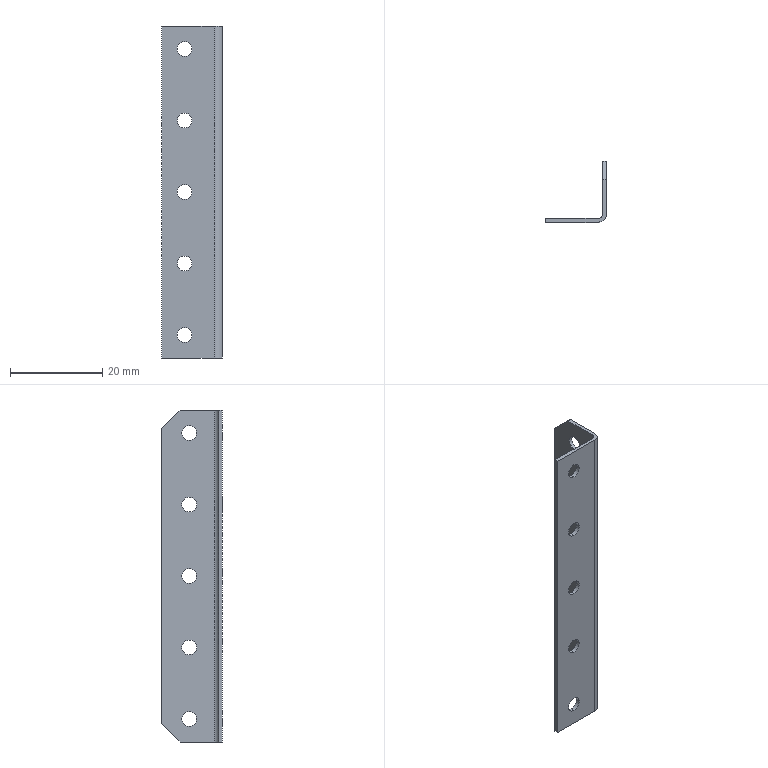Part | SolidWorks | features BaseBody 1 | 1 solid | 32 faces | box 13.2 x 13.2 x 72 mm | volume 1363 mm3 | cylinder 22 | plane 10 | commonest cylinder face diameters 3.2 x20 2 x1 3.6 x1
STEP:
#1=CARTESIAN_POINT('',(-7.5,-0.8,32.6));
#2=VERTEX_POINT('',#1);
#3=CARTESIAN_POINT('',(-7.5,-0.8,29.4));
#4=VERTEX_POINT('',#3);
#5=CARTESIAN_POINT('',(-7.5,-0.8,31.));
#6=DIRECTION('',(0.,-1.,0.));
#7=DIRECTION('',(0.,0.,1.));
#8=AXIS2_PLACEMENT_3D('',#5,#6,#7);
#9=CIRCLE('',#8,1.6);
#10=EDGE_CURVE('',#2,#4,#9,.T.);
#11=ORIENTED_EDGE('',*,*,#10,.T.);
#12=CARTESIAN_POINT('',(-7.5,0.,29.4));
#13=VERTEX_POINT('',#12);
#14=CARTESIAN_POINT('',(-7.5,-0.8,29.4));
#15=DIRECTION('',(0.,1.,0.));
#16=VECTOR('',#15,1000.);
#17=LINE('',#14,#16);
#18=EDGE_CURVE('',#4,#13,#17,.T.);
#19=ORIENTED_EDGE('',*,*,#18,.T.);
#20=CARTESIAN_POINT('',(-7.5,0.,32.6));
#21=VERTEX_POINT('',#20);
#22=CARTESIAN_POINT('',(-7.5,0.,31.));
#23=DIRECTION('',(0.,1.,0.));
#24=DIRECTION('',(0.,0.,1.));
#25=AXIS2_PLACEMENT_3D('',#22,#23,#24);
#26=CIRCLE('',#25,1.6);
#27=EDGE_CURVE('',#13,#21,#26,.T.);
#28=ORIENTED_EDGE('',*,*,#27,.T.);
#29=CARTESIAN_POINT('',(-7.5,-0.8,32.6));
#30=DIRECTION('',(0.,1.,0.));
#31=VECTOR('',#30,1000.);
#32=LINE('',#29,#31);
#33=EDGE_CURVE('',#2,#21,#32,.T.);
#34=ORIENTED_EDGE('',*,*,#33,.F.);
#35=EDGE_LOOP('',(#11,#19,#28,#34));
#36=FACE_OUTER_BOUND('',#35,.T.);
#37=CARTESIAN_POINT('',(-7.5,-0.8,31.));
#38=DIRECTION('',(0.,1.,0.));
#39=DIRECTION('',(0.,0.,1.));
#40=AXIS2_PLACEMENT_3D('',#37,#38,#39);
#41=CYLINDRICAL_SURFACE('',#40,1.6);
#42=ADVANCED_FACE('',(#36),#41,.F.);
#43=CARTESIAN_POINT('',(-7.5,-0.8,-32.6));
#44=VERTEX_POINT('',#43);
#45=CARTESIAN_POINT('',(-7.5,-0.8,-29.4));
#46=VERTEX_POINT('',#45);
#47=CARTESIAN_POINT('',(-7.5,-0.8,-31.));
#48=DIRECTION('',(0.,1.,0.));
#49=DIRECTION('',(0.,0.,1.));
#50=AXIS2_PLACEMENT_3D('',#47,#48,#49);
#51=CIRCLE('',#50,1.6);
#52=EDGE_CURVE('',#44,#46,#51,.T.);
#53=ORIENTED_EDGE('',*,*,#52,.F.);
#54=CARTESIAN_POINT('',(-7.5,0.,-32.6));
#55=VERTEX_POINT('',#54);
#56=CARTESIAN_POINT('',(-7.5,-0.8,-32.6));
#57=DIRECTION('',(0.,1.,0.));
#58=VECTOR('',#57,1000.);
#59=LINE('',#56,#58);
#60=EDGE_CURVE('',#44,#55,#59,.T.);
#61=ORIENTED_EDGE('',*,*,#60,.T.);
#62=CARTESIAN_POINT('',(-7.5,0.,-29.4));
#63=VERTEX_POINT('',#62);
#64=CARTESIAN_POINT('',(-7.5,0.,-31.));
#65=DIRECTION('',(0.,1.,0.));
#66=DIRECTION('',(0.,0.,1.));
#67=AXIS2_PLACEMENT_3D('',#64,#65,#66);
#68=CIRCLE('',#67,1.6);
#69=EDGE_CURVE('',#55,#63,#68,.T.);
#70=ORIENTED_EDGE('',*,*,#69,.T.);
#71=CARTESIAN_POINT('',(-7.5,-0.8,-29.4));
#72=DIRECTION('',(0.,1.,0.));
#73=VECTOR('',#72,1000.);
#74=LINE('',#71,#73);
#75=EDGE_CURVE('',#46,#63,#74,.T.);
#76=ORIENTED_EDGE('',*,*,#75,.F.);
#77=EDGE_LOOP('',(#53,#61,#70,#76));
#78=FACE_OUTER_BOUND('',#77,.T.);
#79=CARTESIAN_POINT('',(-7.5,-0.8,-31.));
#80=DIRECTION('',(0.,1.,0.));
#81=DIRECTION('',(0.,0.,1.));
#82=AXIS2_PLACEMENT_3D('',#79,#80,#81);
#83=CYLINDRICAL_SURFACE('',#82,1.6);
#84=ADVANCED_FACE('',(#78),#83,.F.);
#85=CARTESIAN_POINT('',(-7.5,-0.8,-1.6));
#86=VERTEX_POINT('',#85);
#87=CARTESIAN_POINT('',(-7.5,-0.8,1.6));
#88=VERTEX_POINT('',#87);
#89=CARTESIAN_POINT('',(-7.5,-0.8,0.));
#90=DIRECTION('',(0.,1.,0.));
#91=DIRECTION('',(0.,0.,1.));
#92=AXIS2_PLACEMENT_3D('',#89,#90,#91);
#93=CIRCLE('',#92,1.6);
#94=EDGE_CURVE('',#86,#88,#93,.T.);
#95=ORIENTED_EDGE('',*,*,#94,.F.);
#96=CARTESIAN_POINT('',(-7.5,0.,-1.6));
#97=VERTEX_POINT('',#96);
#98=CARTESIAN_POINT('',(-7.5,-0.8,-1.6));
#99=DIRECTION('',(0.,1.,0.));
#100=VECTOR('',#99,1000.);
#101=LINE('',#98,#100);
#102=EDGE_CURVE('',#86,#97,#101,.T.);
#103=ORIENTED_EDGE('',*,*,#102,.T.);
#104=CARTESIAN_POINT('',(-7.5,0.,1.6));
#105=VERTEX_POINT('',#104);
#106=CARTESIAN_POINT('',(-7.5,0.,0.));
#107=DIRECTION('',(0.,1.,0.));
#108=DIRECTION('',(0.,0.,1.));
#109=AXIS2_PLACEMENT_3D('',#106,#107,#108);
#110=CIRCLE('',#109,1.6);
#111=EDGE_CURVE('',#97,#105,#110,.T.);
#112=ORIENTED_EDGE('',*,*,#111,.T.);
#113=CARTESIAN_POINT('',(-7.5,-0.8,1.6));
#114=DIRECTION('',(0.,1.,0.));
#115=VECTOR('',#114,1000.);
#116=LINE('',#113,#115);
#117=EDGE_CURVE('',#88,#105,#116,.T.);
#118=ORIENTED_EDGE('',*,*,#117,.F.);
#119=EDGE_LOOP('',(#95,#103,#112,#118));
#120=FACE_OUTER_BOUND('',#119,.T.);
#121=CARTESIAN_POINT('',(-7.5,-0.8,0.));
#122=DIRECTION('',(0.,1.,0.));
#123=DIRECTION('',(0.,0.,1.));
#124=AXIS2_PLACEMENT_3D('',#121,#122,#123);
#125=CYLINDRICAL_SURFACE('',#124,1.6);
#126=ADVANCED_FACE('',(#120),#125,.F.);
#127=CARTESIAN_POINT('',(-7.5,-0.8,-17.1));
#128=VERTEX_POINT('',#127);
#129=CARTESIAN_POINT('',(-7.5,-0.8,-13.9));
#130=VERTEX_POINT('',#129);
#131=CARTESIAN_POINT('',(-7.5,-0.8,-15.5));
#132=DIRECTION('',(0.,1.,0.));
#133=DIRECTION('',(0.,0.,1.));
#134=AXIS2_PLACEMENT_3D('',#131,#132,#133);
#135=CIRCLE('',#134,1.6);
#136=EDGE_CURVE('',#128,#130,#135,.T.);
#137=ORIENTED_EDGE('',*,*,#136,.F.);
#138=CARTESIAN_POINT('',(-7.5,0.,-17.1));
#139=VERTEX_POINT('',#138);
#140=CARTESIAN_POINT('',(-7.5,-0.8,-17.1));
#141=DIRECTION('',(0.,1.,0.));
#142=VECTOR('',#141,1000.);
#143=LINE('',#140,#142);
#144=EDGE_CURVE('',#128,#139,#143,.T.);
#145=ORIENTED_EDGE('',*,*,#144,.T.);
#146=CARTESIAN_POINT('',(-7.5,0.,-13.9));
#147=VERTEX_POINT('',#146);
#148=CARTESIAN_POINT('',(-7.5,0.,-15.5));
#149=DIRECTION('',(0.,1.,0.));
#150=DIRECTION('',(0.,0.,1.));
#151=AXIS2_PLACEMENT_3D('',#148,#149,#150);
#152=CIRCLE('',#151,1.6);
#153=EDGE_CURVE('',#139,#147,#152,.T.);
#154=ORIENTED_EDGE('',*,*,#153,.T.);
#155=CARTESIAN_POINT('',(-7.5,-0.8,-13.9));
#156=DIRECTION('',(0.,1.,0.));
#157=VECTOR('',#156,1000.);
#158=LINE('',#155,#157);
#159=EDGE_CURVE('',#130,#147,#158,.T.);
#160=ORIENTED_EDGE('',*,*,#159,.F.);
#161=EDGE_LOOP('',(#137,#145,#154,#160));
#162=FACE_OUTER_BOUND('',#161,.T.);
#163=CARTESIAN_POINT('',(-7.5,-0.8,-15.5));
#164=DIRECTION('',(0.,1.,0.));
#165=DIRECTION('',(0.,0.,1.));
#166=AXIS2_PLACEMENT_3D('',#163,#164,#165);
#167=CYLINDRICAL_SURFACE('',#166,1.6);
#168=ADVANCED_FACE('',(#162),#167,.F.);
#169=CARTESIAN_POINT('',(-7.5,-0.8,13.9));
#170=VERTEX_POINT('',#169);
#171=CARTESIAN_POINT('',(-7.5,-0.8,17.1));
#172=VERTEX_POINT('',#171);
#173=CARTESIAN_POINT('',(-7.5,-0.8,15.5));
#174=DIRECTION('',(0.,1.,0.));
#175=DIRECTION('',(0.,0.,1.));
#176=AXIS2_PLACEMENT_3D('',#173,#174,#175);
#177=CIRCLE('',#176,1.6);
#178=EDGE_CURVE('',#170,#172,#177,.T.);
#179=ORIENTED_EDGE('',*,*,#178,.F.);
#180=CARTESIAN_POINT('',(-7.5,0.,13.9));
#181=VERTEX_POINT('',#180);
#182=CARTESIAN_POINT('',(-7.5,-0.8,13.9));
#183=DIRECTION('',(0.,1.,0.));
#184=VECTOR('',#183,1000.);
#185=LINE('',#182,#184);
#186=EDGE_CURVE('',#170,#181,#185,.T.);
#187=ORIENTED_EDGE('',*,*,#186,.T.);
#188=CARTESIAN_POINT('',(-7.5,0.,17.1));
#189=VERTEX_POINT('',#188);
#190=CARTESIAN_POINT('',(-7.5,0.,15.5));
#191=DIRECTION('',(0.,1.,0.));
#192=DIRECTION('',(0.,0.,1.));
#193=AXIS2_PLACEMENT_3D('',#190,#191,#192);
#194=CIRCLE('',#193,1.6);
#195=EDGE_CURVE('',#181,#189,#194,.T.);
#196=ORIENTED_EDGE('',*,*,#195,.T.);
#197=CARTESIAN_POINT('',(-7.5,-0.8,17.1));
#198=DIRECTION('',(0.,1.,0.));
#199=VECTOR('',#198,1000.);
#200=LINE('',#197,#199);
#201=EDGE_CURVE('',#172,#189,#200,.T.);
#202=ORIENTED_EDGE('',*,*,#201,.F.);
#203=EDGE_LOOP('',(#179,#187,#196,#202));
#204=FACE_OUTER_BOUND('',#203,.T.);
#205=CARTESIAN_POINT('',(-7.5,-0.8,15.5));
#206=DIRECTION('',(0.,1.,0.));
#207=DIRECTION('',(0.,0.,1.));
#208=AXIS2_PLACEMENT_3D('',#205,#206,#207);
#209=CYLINDRICAL_SURFACE('',#208,1.6);
#210=ADVANCED_FACE('',(#204),#209,.F.);
#211=CARTESIAN_POINT('',(0.7004,6.4,-32.6));
#212=VERTEX_POINT('',#211);
#213=CARTESIAN_POINT('',(0.7004,6.4,-29.4));
#214=VERTEX_POINT('',#213);
#215=CARTESIAN_POINT('',(0.7004,6.4,-31.));
#216=DIRECTION('',(-1.,0.,0.));
#217=DIRECTION('',(0.,0.,1.));
#218=AXIS2_PLACEMENT_3D('',#215,#216,#217);
#219=CIRCLE('',#218,1.6);
#220=EDGE_CURVE('',#212,#214,#219,.T.);
#221=ORIENTED_EDGE('',*,*,#220,.F.);
#222=CARTESIAN_POINT('',(-0.09956,6.4,-32.6));
#223=VERTEX_POINT('',#222);
#224=CARTESIAN_POINT('',(0.7004,6.4,-32.6));
#225=DIRECTION('',(-1.,0.,0.));
#226=VECTOR('',#225,1000.);
#227=LINE('',#224,#226);
#228=EDGE_CURVE('',#212,#223,#227,.T.);
#229=ORIENTED_EDGE('',*,*,#228,.T.);
#230=CARTESIAN_POINT('',(-0.09956,6.4,-29.4));
#231=VERTEX_POINT('',#230);
#232=CARTESIAN_POINT('',(-0.09956,6.4,-31.));
#233=DIRECTION('',(-1.,0.,0.));
#234=DIRECTION('',(0.,0.,1.));
#235=AXIS2_PLACEMENT_3D('',#232,#233,#234);
#236=CIRCLE('',#235,1.6);
#237=EDGE_CURVE('',#223,#231,#236,.T.);
#238=ORIENTED_EDGE('',*,*,#237,.T.);
#239=CARTESIAN_POINT('',(0.7004,6.4,-29.4));
#240=DIRECTION('',(-1.,0.,0.));
#241=VECTOR('',#240,1000.);
#242=LINE('',#239,#241);
#243=EDGE_CURVE('',#214,#231,#242,.T.);
#244=ORIENTED_EDGE('',*,*,#243,.F.);
#245=EDGE_LOOP('',(#221,#229,#238,#244));
#246=FACE_OUTER_BOUND('',#245,.T.);
#247=CARTESIAN_POINT('',(0.7004,6.4,-31.));
#248=DIRECTION('',(-1.,0.,0.));
#249=DIRECTION('',(0.,0.,1.));
#250=AXIS2_PLACEMENT_3D('',#247,#248,#249);
#251=CYLINDRICAL_SURFACE('',#250,1.6);
#252=ADVANCED_FACE('',(#246),#251,.F.);
#253=CARTESIAN_POINT('',(0.7004,6.4,29.4));
#254=VERTEX_POINT('',#253);
#255=CARTESIAN_POINT('',(0.7004,6.4,32.6));
#256=VERTEX_POINT('',#255);
#257=CARTESIAN_POINT('',(0.7004,6.4,31.));
#258=DIRECTION('',(-1.,0.,0.));
#259=DIRECTION('',(0.,0.,1.));
#260=AXIS2_PLACEMENT_3D('',#257,#258,#259);
#261=CIRCLE('',#260,1.6);
#262=EDGE_CURVE('',#254,#256,#261,.T.);
#263=ORIENTED_EDGE('',*,*,#262,.F.);
#264=CARTESIAN_POINT('',(-0.09956,6.4,29.4));
#265=VERTEX_POINT('',#264);
#266=CARTESIAN_POINT('',(0.7004,6.4,29.4));
#267=DIRECTION('',(-1.,0.,0.));
#268=VECTOR('',#267,1000.);
#269=LINE('',#266,#268);
#270=EDGE_CURVE('',#254,#265,#269,.T.);
#271=ORIENTED_EDGE('',*,*,#270,.T.);
#272=CARTESIAN_POINT('',(-0.09956,6.4,32.6));
#273=VERTEX_POINT('',#272);
#274=CARTESIAN_POINT('',(-0.09956,6.4,31.));
#275=DIRECTION('',(-1.,0.,0.));
#276=DIRECTION('',(0.,0.,1.));
#277=AXIS2_PLACEMENT_3D('',#274,#275,#276);
#278=CIRCLE('',#277,1.6);
#279=EDGE_CURVE('',#265,#273,#278,.T.);
#280=ORIENTED_EDGE('',*,*,#279,.T.);
#281=CARTESIAN_POINT('',(0.7004,6.4,32.6));
#282=DIRECTION('',(-1.,0.,0.));
#283=VECTOR('',#282,1000.);
#284=LINE('',#281,#283);
#285=EDGE_CURVE('',#256,#273,#284,.T.);
#286=ORIENTED_EDGE('',*,*,#285,.F.);
#287=EDGE_LOOP('',(#263,#271,#280,#286));
#288=FACE_OUTER_BOUND('',#287,.T.);
#289=CARTESIAN_POINT('',(0.7004,6.4,31.));
#290=DIRECTION('',(-1.,0.,0.));
#291=DIRECTION('',(0.,0.,1.));
#292=AXIS2_PLACEMENT_3D('',#289,#290,#291);
#293=CYLINDRICAL_SURFACE('',#292,1.6);
#294=ADVANCED_FACE('',(#288),#293,.F.);
#295=CARTESIAN_POINT('',(0.7004,6.4,-1.6));
#296=VERTEX_POINT('',#295);
#297=CARTESIAN_POINT('',(0.7004,6.4,1.6));
#298=VERTEX_POINT('',#297);
#299=CARTESIAN_POINT('',(0.7004,6.4,0.));
#300=DIRECTION('',(-1.,0.,0.));
#301=DIRECTION('',(0.,0.,1.));
#302=AXIS2_PLACEMENT_3D('',#299,#300,#301);
#303=CIRCLE('',#302,1.6);
#304=EDGE_CURVE('',#296,#298,#303,.T.);
#305=ORIENTED_EDGE('',*,*,#304,.F.);
#306=CARTESIAN_POINT('',(-0.09956,6.4,-1.6));
#307=VERTEX_POINT('',#306);
#308=CARTESIAN_POINT('',(0.7004,6.4,-1.6));
#309=DIRECTION('',(-1.,0.,0.));
#310=VECTOR('',#309,1000.);
#311=LINE('',#308,#310);
#312=EDGE_CURVE('',#296,#307,#311,.T.);
#313=ORIENTED_EDGE('',*,*,#312,.T.);
#314=CARTESIAN_POINT('',(-0.09956,6.4,1.6));
#315=VERTEX_POINT('',#314);
#316=CARTESIAN_POINT('',(-0.09956,6.4,0.));
#317=DIRECTION('',(-1.,0.,0.));
#318=DIRECTION('',(0.,0.,1.));
#319=AXIS2_PLACEMENT_3D('',#316,#317,#318);
#320=CIRCLE('',#319,1.6);
#321=EDGE_CURVE('',#307,#315,#320,.T.);
#322=ORIENTED_EDGE('',*,*,#321,.T.);
#323=CARTESIAN_POINT('',(0.7004,6.4,1.6));
#324=DIRECTION('',(-1.,0.,0.));
#325=VECTOR('',#324,1000.);
#326=LINE('',#323,#325);
#327=EDGE_CURVE('',#298,#315,#326,.T.);
#328=ORIENTED_EDGE('',*,*,#327,.F.);
#329=EDGE_LOOP('',(#305,#313,#322,#328));
#330=FACE_OUTER_BOUND('',#329,.T.);
#331=CARTESIAN_POINT('',(0.7004,6.4,0.));
#332=DIRECTION('',(-1.,0.,0.));
#333=DIRECTION('',(0.,0.,1.));
#334=AXIS2_PLACEMENT_3D('',#331,#332,#333);
#335=CYLINDRICAL_SURFACE('',#334,1.6);
#336=ADVANCED_FACE('',(#330),#335,.F.);
#337=CARTESIAN_POINT('',(0.7004,6.4,13.9));
#338=VERTEX_POINT('',#337);
#339=CARTESIAN_POINT('',(0.7004,6.4,17.1));
#340=VERTEX_POINT('',#339);
#341=CARTESIAN_POINT('',(0.7004,6.4,15.5));
#342=DIRECTION('',(-1.,0.,0.));
#343=DIRECTION('',(0.,0.,1.));
#344=AXIS2_PLACEMENT_3D('',#341,#342,#343);
#345=CIRCLE('',#344,1.6);
#346=EDGE_CURVE('',#338,#340,#345,.T.);
#347=ORIENTED_EDGE('',*,*,#346,.F.);
#348=CARTESIAN_POINT('',(-0.09956,6.4,13.9));
#349=VERTEX_POINT('',#348);
#350=CARTESIAN_POINT('',(0.7004,6.4,13.9));
#351=DIRECTION('',(-1.,0.,0.));
#352=VECTOR('',#351,1000.);
#353=LINE('',#350,#352);
#354=EDGE_CURVE('',#338,#349,#353,.T.);
#355=ORIENTED_EDGE('',*,*,#354,.T.);
#356=CARTESIAN_POINT('',(-0.09956,6.4,17.1));
#357=VERTEX_POINT('',#356);
#358=CARTESIAN_POINT('',(-0.09956,6.4,15.5));
#359=DIRECTION('',(-1.,0.,0.));
#360=DIRECTION('',(0.,0.,1.));
#361=AXIS2_PLACEMENT_3D('',#358,#359,#360);
#362=CIRCLE('',#361,1.6);
#363=EDGE_CURVE('',#349,#357,#362,.T.);
#364=ORIENTED_EDGE('',*,*,#363,.T.);
#365=CARTESIAN_POINT('',(0.7004,6.4,17.1));
#366=DIRECTION('',(-1.,0.,0.));
#367=VECTOR('',#366,1000.);
#368=LINE('',#365,#367);
#369=EDGE_CURVE('',#340,#357,#368,.T.);
#370=ORIENTED_EDGE('',*,*,#369,.F.);
#371=EDGE_LOOP('',(#347,#355,#364,#370));
#372=FACE_OUTER_BOUND('',#371,.T.);
#373=CARTESIAN_POINT('',(0.7004,6.4,15.5));
#374=DIRECTION('',(-1.,0.,0.));
#375=DIRECTION('',(0.,0.,1.));
#376=AXIS2_PLACEMENT_3D('',#373,#374,#375);
#377=CYLINDRICAL_SURFACE('',#376,1.6);
#378=ADVANCED_FACE('',(#372),#377,.F.);
#379=CARTESIAN_POINT('',(0.7004,6.4,-17.1));
#380=VERTEX_POINT('',#379);
#381=CARTESIAN_POINT('',(0.7004,6.4,-13.9));
#382=VERTEX_POINT('',#381);
#383=CARTESIAN_POINT('',(0.7004,6.4,-15.5));
#384=DIRECTION('',(-1.,0.,0.));
#385=DIRECTION('',(0.,0.,1.));
#386=AXIS2_PLACEMENT_3D('',#383,#384,#385);
#387=CIRCLE('',#386,1.6);
#388=EDGE_CURVE('',#380,#382,#387,.T.);
#389=ORIENTED_EDGE('',*,*,#388,.F.);
#390=CARTESIAN_POINT('',(-0.09956,6.4,-17.1));
#391=VERTEX_POINT('',#390);
#392=CARTESIAN_POINT('',(0.7004,6.4,-17.1));
#393=DIRECTION('',(-1.,0.,0.));
#394=VECTOR('',#393,1000.);
#395=LINE('',#392,#394);
#396=EDGE_CURVE('',#380,#391,#395,.T.);
#397=ORIENTED_EDGE('',*,*,#396,.T.);
#398=CARTESIAN_POINT('',(-0.09956,6.4,-13.9));
#399=VERTEX_POINT('',#398);
#400=CARTESIAN_POINT('',(-0.09956,6.4,-15.5));
#401=DIRECTION('',(-1.,0.,0.));
#402=DIRECTION('',(0.,0.,1.));
#403=AXIS2_PLACEMENT_3D('',#400,#401,#402);
#404=CIRCLE('',#403,1.6);
#405=EDGE_CURVE('',#391,#399,#404,.T.);
#406=ORIENTED_EDGE('',*,*,#405,.T.);
#407=CARTESIAN_POINT('',(0.7004,6.4,-13.9));
#408=DIRECTION('',(-1.,0.,0.));
#409=VECTOR('',#408,1000.);
#410=LINE('',#407,#409);
#411=EDGE_CURVE('',#382,#399,#410,.T.);
#412=ORIENTED_EDGE('',*,*,#411,.F.);
#413=EDGE_LOOP('',(#389,#397,#406,#412));
#414=FACE_OUTER_BOUND('',#413,.T.);
#415=CARTESIAN_POINT('',(0.7004,6.4,-15.5));
#416=DIRECTION('',(-1.,0.,0.));
#417=DIRECTION('',(0.,0.,1.));
#418=AXIS2_PLACEMENT_3D('',#415,#416,#417);
#419=CYLINDRICAL_SURFACE('',#418,1.6);
#420=ADVANCED_FACE('',(#414),#419,.F.);
#421=ORIENTED_EDGE('',*,*,#18,.F.);
#422=CARTESIAN_POINT('',(-7.5,-0.8,31.));
#423=DIRECTION('',(0.,-1.,0.));
#424=DIRECTION('',(0.,0.,1.));
#425=AXIS2_PLACEMENT_3D('',#422,#423,#424);
#426=CIRCLE('',#425,1.6);
#427=EDGE_CURVE('',#4,#2,#426,.T.);
#428=ORIENTED_EDGE('',*,*,#427,.T.);
#429=ORIENTED_EDGE('',*,*,#33,.T.);
#430=CARTESIAN_POINT('',(-7.5,0.,31.));
#431=DIRECTION('',(0.,1.,0.));
#432=DIRECTION('',(0.,0.,1.));
#433=AXIS2_PLACEMENT_3D('',#430,#431,#432);
#434=CIRCLE('',#433,1.6);
#435=EDGE_CURVE('',#21,#13,#434,.T.);
#436=ORIENTED_EDGE('',*,*,#435,.T.);
#437=EDGE_LOOP('',(#421,#428,#429,#436));
#438=FACE_OUTER_BOUND('',#437,.T.);
#439=CARTESIAN_POINT('',(-7.5,-0.8,31.));
#440=DIRECTION('',(0.,1.,0.));
#441=DIRECTION('',(0.,0.,1.));
#442=AXIS2_PLACEMENT_3D('',#439,#440,#441);
#443=CYLINDRICAL_SURFACE('',#442,1.6);
#444=ADVANCED_FACE('',(#438),#443,.F.);
#445=CARTESIAN_POINT('',(-7.5,0.,-31.));
#446=DIRECTION('',(0.,1.,0.));
#447=DIRECTION('',(0.,0.,1.));
#448=AXIS2_PLACEMENT_3D('',#445,#446,#447);
#449=CIRCLE('',#448,1.6);
#450=EDGE_CURVE('',#63,#55,#449,.T.);
#451=ORIENTED_EDGE('',*,*,#450,.F.);
#452=ORIENTED_EDGE('',*,*,#69,.F.);
#453=EDGE_LOOP('',(#451,#452));
#454=FACE_BOUND('',#453,.T.);
#455=CARTESIAN_POINT('',(-7.5,0.,0.));
#456=DIRECTION('',(0.,1.,0.));
#457=DIRECTION('',(0.,0.,1.));
#458=AXIS2_PLACEMENT_3D('',#455,#456,#457);
#459=CIRCLE('',#458,1.6);
#460=EDGE_CURVE('',#105,#97,#459,.T.);
#461=ORIENTED_EDGE('',*,*,#460,.F.);
#462=ORIENTED_EDGE('',*,*,#111,.F.);
#463=EDGE_LOOP('',(#461,#462));
#464=FACE_BOUND('',#463,.T.);
#465=CARTESIAN_POINT('',(-7.5,0.,-15.5));
#466=DIRECTION('',(0.,1.,0.));
#467=DIRECTION('',(0.,0.,1.));
#468=AXIS2_PLACEMENT_3D('',#465,#466,#467);
#469=CIRCLE('',#468,1.6);
#470=EDGE_CURVE('',#147,#139,#469,.T.);
#471=ORIENTED_EDGE('',*,*,#470,.F.);
#472=ORIENTED_EDGE('',*,*,#153,.F.);
#473=EDGE_LOOP('',(#471,#472));
#474=FACE_BOUND('',#473,.T.);
#475=CARTESIAN_POINT('',(-7.5,0.,15.5));
#476=DIRECTION('',(0.,1.,0.));
#477=DIRECTION('',(0.,0.,1.));
#478=AXIS2_PLACEMENT_3D('',#475,#476,#477);
#479=CIRCLE('',#478,1.6);
#480=EDGE_CURVE('',#189,#181,#479,.T.);
#481=ORIENTED_EDGE('',*,*,#480,.F.);
#482=ORIENTED_EDGE('',*,*,#195,.F.);
#483=EDGE_LOOP('',(#481,#482));
#484=FACE_BOUND('',#483,.T.);
#485=ORIENTED_EDGE('',*,*,#435,.F.);
#486=ORIENTED_EDGE('',*,*,#27,.F.);
#487=EDGE_LOOP('',(#485,#486));
#488=FACE_BOUND('',#487,.T.);
#489=CARTESIAN_POINT('',(-12.5,0.,-36.));
#490=VERTEX_POINT('',#489);
#491=CARTESIAN_POINT('',(-1.1,0.,-36.));
#492=VERTEX_POINT('',#491);
#493=CARTESIAN_POINT('',(-6.8,0.,-36.));
#494=DIRECTION('',(1.,0.,0.));
#495=VECTOR('',#494,1000.);
#496=LINE('',#493,#495);
#497=EDGE_CURVE('',#490,#492,#496,.T.);
#498=ORIENTED_EDGE('',*,*,#497,.F.);
#499=CARTESIAN_POINT('',(-12.5,0.,36.));
#500=VERTEX_POINT('',#499);
#501=CARTESIAN_POINT('',(-12.5,0.,0.));
#502=DIRECTION('',(0.,0.,-1.));
#503=VECTOR('',#502,1000.);
#504=LINE('',#501,#503);
#505=EDGE_CURVE('',#500,#490,#504,.T.);
#506=ORIENTED_EDGE('',*,*,#505,.F.);
#507=CARTESIAN_POINT('',(-1.1,0.,36.));
#508=VERTEX_POINT('',#507);
#509=CARTESIAN_POINT('',(-6.8,0.,36.));
#510=DIRECTION('',(-1.,0.,0.));
#511=VECTOR('',#510,1000.);
#512=LINE('',#509,#511);
#513=EDGE_CURVE('',#508,#500,#512,.T.);
#514=ORIENTED_EDGE('',*,*,#513,.F.);
#515=CARTESIAN_POINT('',(-1.1,0.,0.));
#516=DIRECTION('',(0.,0.,1.));
#517=VECTOR('',#516,1000.);
#518=LINE('',#515,#517);
#519=EDGE_CURVE('',#492,#508,#518,.T.);
#520=ORIENTED_EDGE('',*,*,#519,.F.);
#521=EDGE_LOOP('',(#498,#506,#514,#520));
#522=FACE_OUTER_BOUND('',#521,.T.);
#523=CARTESIAN_POINT('',(-12.5,0.,36.));
#524=DIRECTION('',(0.,-1.,0.));
#525=DIRECTION('',(0.,0.,-1.));
#526=AXIS2_PLACEMENT_3D('',#523,#524,#525);
#527=PLANE('',#526);
#528=ADVANCED_FACE('',(#454,#464,#474,#484,#488,#522),#527,.F.);
#529=CARTESIAN_POINT('',(-7.5,-0.8,-31.));
#530=DIRECTION('',(0.,1.,0.));
#531=DIRECTION('',(0.,0.,1.));
#532=AXIS2_PLACEMENT_3D('',#529,#530,#531);
#533=CIRCLE('',#532,1.6);
#534=EDGE_CURVE('',#46,#44,#533,.T.);
#535=ORIENTED_EDGE('',*,*,#534,.T.);
#536=ORIENTED_EDGE('',*,*,#52,.T.);
#537=EDGE_LOOP('',(#535,#536));
#538=FACE_BOUND('',#537,.T.);
#539=CARTESIAN_POINT('',(-7.5,-0.8,0.));
#540=DIRECTION('',(0.,1.,0.));
#541=DIRECTION('',(0.,0.,1.));
#542=AXIS2_PLACEMENT_3D('',#539,#540,#541);
#543=CIRCLE('',#542,1.6);
#544=EDGE_CURVE('',#88,#86,#543,.T.);
#545=ORIENTED_EDGE('',*,*,#544,.T.);
#546=ORIENTED_EDGE('',*,*,#94,.T.);
#547=EDGE_LOOP('',(#545,#546));
#548=FACE_BOUND('',#547,.T.);
#549=CARTESIAN_POINT('',(-7.5,-0.8,-15.5));
#550=DIRECTION('',(0.,1.,0.));
#551=DIRECTION('',(0.,0.,1.));
#552=AXIS2_PLACEMENT_3D('',#549,#550,#551);
#553=CIRCLE('',#552,1.6);
#554=EDGE_CURVE('',#130,#128,#553,.T.);
#555=ORIENTED_EDGE('',*,*,#554,.T.);
#556=ORIENTED_EDGE('',*,*,#136,.T.);
#557=EDGE_LOOP('',(#555,#556));
#558=FACE_BOUND('',#557,.T.);
#559=CARTESIAN_POINT('',(-7.5,-0.8,15.5));
#560=DIRECTION('',(0.,1.,0.));
#561=DIRECTION('',(0.,0.,1.));
#562=AXIS2_PLACEMENT_3D('',#559,#560,#561);
#563=CIRCLE('',#562,1.6);
#564=EDGE_CURVE('',#172,#170,#563,.T.);
#565=ORIENTED_EDGE('',*,*,#564,.T.);
#566=ORIENTED_EDGE('',*,*,#178,.T.);
#567=EDGE_LOOP('',(#565,#566));
#568=FACE_BOUND('',#567,.T.);
#569=ORIENTED_EDGE('',*,*,#10,.F.);
#570=ORIENTED_EDGE('',*,*,#427,.F.);
#571=EDGE_LOOP('',(#569,#570));
#572=FACE_BOUND('',#571,.T.);
#573=CARTESIAN_POINT('',(-1.1,-0.8,36.));
#574=VERTEX_POINT('',#573);
#575=CARTESIAN_POINT('',(-12.5,-0.8,36.));
#576=VERTEX_POINT('',#575);
#577=CARTESIAN_POINT('',(-6.8,-0.8,36.));
#578=DIRECTION('',(-1.,0.,0.));
#579=VECTOR('',#578,1000.);
#580=LINE('',#577,#579);
#581=EDGE_CURVE('',#574,#576,#580,.T.);
#582=ORIENTED_EDGE('',*,*,#581,.T.);
#583=CARTESIAN_POINT('',(-12.5,-0.8,-36.));
#584=VERTEX_POINT('',#583);
#585=CARTESIAN_POINT('',(-12.5,-0.8,0.));
#586=DIRECTION('',(0.,0.,-1.));
#587=VECTOR('',#586,1000.);
#588=LINE('',#585,#587);
#589=EDGE_CURVE('',#576,#584,#588,.T.);
#590=ORIENTED_EDGE('',*,*,#589,.T.);
#591=CARTESIAN_POINT('',(-1.1,-0.8,-36.));
#592=VERTEX_POINT('',#591);
#593=CARTESIAN_POINT('',(-6.8,-0.8,-36.));
#594=DIRECTION('',(1.,0.,0.));
#595=VECTOR('',#594,1000.);
#596=LINE('',#593,#595);
#597=EDGE_CURVE('',#584,#592,#596,.T.);
#598=ORIENTED_EDGE('',*,*,#597,.T.);
#599=CARTESIAN_POINT('',(-1.1,-0.8,0.));
#600=DIRECTION('',(0.,0.,1.));
#601=VECTOR('',#600,1000.);
#602=LINE('',#599,#601);
#603=EDGE_CURVE('',#592,#574,#602,.T.);
#604=ORIENTED_EDGE('',*,*,#603,.T.);
#605=EDGE_LOOP('',(#582,#590,#598,#604));
#606=FACE_OUTER_BOUND('',#605,.T.);
#607=CARTESIAN_POINT('',(-12.5,-0.8,36.));
#608=DIRECTION('',(0.,-1.,0.));
#609=DIRECTION('',(0.,0.,-1.));
#610=AXIS2_PLACEMENT_3D('',#607,#608,#609);
#611=PLANE('',#610);
#612=ADVANCED_FACE('',(#538,#548,#558,#568,#572,#606),#611,.T.);
#613=ORIENTED_EDGE('',*,*,#60,.F.);
#614=ORIENTED_EDGE('',*,*,#534,.F.);
#615=ORIENTED_EDGE('',*,*,#75,.T.);
#616=ORIENTED_EDGE('',*,*,#450,.T.);
#617=EDGE_LOOP('',(#613,#614,#615,#616));
#618=FACE_OUTER_BOUND('',#617,.T.);
#619=CARTESIAN_POINT('',(-7.5,-0.8,-31.));
#620=DIRECTION('',(0.,1.,0.));
#621=DIRECTION('',(0.,0.,1.));
#622=AXIS2_PLACEMENT_3D('',#619,#620,#621);
#623=CYLINDRICAL_SURFACE('',#622,1.6);
#624=ADVANCED_FACE('',(#618),#623,.F.);
#625=ORIENTED_EDGE('',*,*,#102,.F.);
#626=ORIENTED_EDGE('',*,*,#544,.F.);
#627=ORIENTED_EDGE('',*,*,#117,.T.);
#628=ORIENTED_EDGE('',*,*,#460,.T.);
#629=EDGE_LOOP('',(#625,#626,#627,#628));
#630=FACE_OUTER_BOUND('',#629,.T.);
#631=CARTESIAN_POINT('',(-7.5,-0.8,0.));
#632=DIRECTION('',(0.,1.,0.));
#633=DIRECTION('',(0.,0.,1.));
#634=AXIS2_PLACEMENT_3D('',#631,#632,#633);
#635=CYLINDRICAL_SURFACE('',#634,1.6);
#636=ADVANCED_FACE('',(#630),#635,.F.);
#637=ORIENTED_EDGE('',*,*,#144,.F.);
#638=ORIENTED_EDGE('',*,*,#554,.F.);
#639=ORIENTED_EDGE('',*,*,#159,.T.);
#640=ORIENTED_EDGE('',*,*,#470,.T.);
#641=EDGE_LOOP('',(#637,#638,#639,#640));
#642=FACE_OUTER_BOUND('',#641,.T.);
#643=CARTESIAN_POINT('',(-7.5,-0.8,-15.5));
#644=DIRECTION('',(0.,1.,0.));
#645=DIRECTION('',(0.,0.,1.));
#646=AXIS2_PLACEMENT_3D('',#643,#644,#645);
#647=CYLINDRICAL_SURFACE('',#646,1.6);
#648=ADVANCED_FACE('',(#642),#647,.F.);
#649=ORIENTED_EDGE('',*,*,#186,.F.);
#650=ORIENTED_EDGE('',*,*,#564,.F.);
#651=ORIENTED_EDGE('',*,*,#201,.T.);
#652=ORIENTED_EDGE('',*,*,#480,.T.);
#653=EDGE_LOOP('',(#649,#650,#651,#652));
#654=FACE_OUTER_BOUND('',#653,.T.);
#655=CARTESIAN_POINT('',(-7.5,-0.8,15.5));
#656=DIRECTION('',(0.,1.,0.));
#657=DIRECTION('',(0.,0.,1.));
#658=AXIS2_PLACEMENT_3D('',#655,#656,#657);
#659=CYLINDRICAL_SURFACE('',#658,1.6);
#660=ADVANCED_FACE('',(#654),#659,.F.);
#661=ORIENTED_EDGE('',*,*,#519,.T.);
#662=CARTESIAN_POINT('',(-0.09956,1.,36.));
#663=VERTEX_POINT('',#662);
#664=CARTESIAN_POINT('',(-1.1,1.,36.));
#665=DIRECTION('',(0.,0.,-1.));
#666=DIRECTION('',(1.,0.,0.));
#667=AXIS2_PLACEMENT_3D('',#664,#665,#666);
#668=CIRCLE('',#667,1.);
#669=EDGE_CURVE('',#663,#508,#668,.T.);
#670=ORIENTED_EDGE('',*,*,#669,.F.);
#671=CARTESIAN_POINT('',(-0.09956,1.,-36.));
#672=VERTEX_POINT('',#671);
#673=CARTESIAN_POINT('',(-0.09956,1.,0.));
#674=DIRECTION('',(0.,0.,-1.));
#675=VECTOR('',#674,1000.);
#676=LINE('',#673,#675);
#677=EDGE_CURVE('',#663,#672,#676,.T.);
#678=ORIENTED_EDGE('',*,*,#677,.T.);
#679=CARTESIAN_POINT('',(-1.1,1.,-36.));
#680=DIRECTION('',(0.,0.,1.));
#681=DIRECTION('',(1.,0.,0.));
#682=AXIS2_PLACEMENT_3D('',#679,#680,#681);
#683=CIRCLE('',#682,1.);
#684=EDGE_CURVE('',#492,#672,#683,.T.);
#685=ORIENTED_EDGE('',*,*,#684,.F.);
#686=EDGE_LOOP('',(#661,#670,#678,#685));
#687=FACE_OUTER_BOUND('',#686,.T.);
#688=CARTESIAN_POINT('',(-1.1,1.,-36.));
#689=DIRECTION('',(0.,0.,1.));
#690=DIRECTION('',(1.,0.,0.));
#691=AXIS2_PLACEMENT_3D('',#688,#689,#690);
#692=CYLINDRICAL_SURFACE('',#691,1.);
#693=ADVANCED_FACE('',(#687),#692,.F.);
#694=ORIENTED_EDGE('',*,*,#597,.F.);
#695=CARTESIAN_POINT('',(-12.5,-0.4,-36.));
#696=DIRECTION('',(0.,1.,0.));
#697=VECTOR('',#696,1000.);
#698=LINE('',#695,#697);
#699=EDGE_CURVE('',#584,#490,#698,.T.);
#700=ORIENTED_EDGE('',*,*,#699,.T.);
#701=ORIENTED_EDGE('',*,*,#497,.T.);
#702=ORIENTED_EDGE('',*,*,#684,.T.);
#703=CARTESIAN_POINT('',(-0.09956,8.4,-36.));
#704=VERTEX_POINT('',#703);
#705=CARTESIAN_POINT('',(-0.09956,6.7,-36.));
#706=DIRECTION('',(0.,1.,0.));
#707=VECTOR('',#706,1000.);
#708=LINE('',#705,#707);
#709=EDGE_CURVE('',#672,#704,#708,.T.);
#710=ORIENTED_EDGE('',*,*,#709,.T.);
#711=CARTESIAN_POINT('',(0.7004,8.4,-36.));
#712=VERTEX_POINT('',#711);
#713=CARTESIAN_POINT('',(0.3004,8.4,-36.));
#714=DIRECTION('',(1.,0.,0.));
#715=VECTOR('',#714,1000.);
#716=LINE('',#713,#715);
#717=EDGE_CURVE('',#704,#712,#716,.T.);
#718=ORIENTED_EDGE('',*,*,#717,.T.);
#719=CARTESIAN_POINT('',(0.7004,1.,-36.));
#720=VERTEX_POINT('',#719);
#721=CARTESIAN_POINT('',(0.7004,6.7,-36.));
#722=DIRECTION('',(0.,1.,0.));
#723=VECTOR('',#722,1000.);
#724=LINE('',#721,#723);
#725=EDGE_CURVE('',#720,#712,#724,.T.);
#726=ORIENTED_EDGE('',*,*,#725,.F.);
#727=CARTESIAN_POINT('',(-1.1,1.,-36.));
#728=DIRECTION('',(0.,0.,-1.));
#729=DIRECTION('',(1.,0.,0.));
#730=AXIS2_PLACEMENT_3D('',#727,#728,#729);
#731=CIRCLE('',#730,1.8);
#732=EDGE_CURVE('',#720,#592,#731,.T.);
#733=ORIENTED_EDGE('',*,*,#732,.T.);
#734=EDGE_LOOP('',(#694,#700,#701,#702,#710,#718,#726,#733));
#735=FACE_OUTER_BOUND('',#734,.T.);
#736=CARTESIAN_POINT('',(-1.1,-0.8,-36.));
#737=DIRECTION('',(0.,0.,-1.));
#738=DIRECTION('',(-1.,0.,0.));
#739=AXIS2_PLACEMENT_3D('',#736,#737,#738);
#740=PLANE('',#739);
#741=ADVANCED_FACE('',(#735),#740,.T.);
#742=ORIENTED_EDGE('',*,*,#589,.F.);
#743=CARTESIAN_POINT('',(-12.5,-0.4,36.));
#744=DIRECTION('',(0.,1.,0.));
#745=VECTOR('',#744,1000.);
#746=LINE('',#743,#745);
#747=EDGE_CURVE('',#576,#500,#746,.T.);
#748=ORIENTED_EDGE('',*,*,#747,.T.);
#749=ORIENTED_EDGE('',*,*,#505,.T.);
#750=ORIENTED_EDGE('',*,*,#699,.F.);
#751=EDGE_LOOP('',(#742,#748,#749,#750));
#752=FACE_OUTER_BOUND('',#751,.T.);
#753=CARTESIAN_POINT('',(-12.5,-0.8,-36.));
#754=DIRECTION('',(-1.,0.,0.));
#755=DIRECTION('',(0.,0.,1.));
#756=AXIS2_PLACEMENT_3D('',#753,#754,#755);
#757=PLANE('',#756);
#758=ADVANCED_FACE('',(#752),#757,.T.);
#759=ORIENTED_EDGE('',*,*,#513,.T.);
#760=ORIENTED_EDGE('',*,*,#747,.F.);
#761=ORIENTED_EDGE('',*,*,#581,.F.);
#762=CARTESIAN_POINT('',(0.7004,1.,36.));
#763=VERTEX_POINT('',#762);
#764=CARTESIAN_POINT('',(-1.1,1.,36.));
#765=DIRECTION('',(0.,0.,1.));
#766=DIRECTION('',(1.,0.,0.));
#767=AXIS2_PLACEMENT_3D('',#764,#765,#766);
#768=CIRCLE('',#767,1.8);
#769=EDGE_CURVE('',#574,#763,#768,.T.);
#770=ORIENTED_EDGE('',*,*,#769,.T.);
#771=CARTESIAN_POINT('',(0.7004,8.4,36.));
#772=VERTEX_POINT('',#771);
#773=CARTESIAN_POINT('',(0.7004,6.7,36.));
#774=DIRECTION('',(0.,-1.,0.));
#775=VECTOR('',#774,1000.);
#776=LINE('',#773,#775);
#777=EDGE_CURVE('',#772,#763,#776,.T.);
#778=ORIENTED_EDGE('',*,*,#777,.F.);
#779=CARTESIAN_POINT('',(-0.09956,8.4,36.));
#780=VERTEX_POINT('',#779);
#781=CARTESIAN_POINT('',(0.3004,8.4,36.));
#782=DIRECTION('',(-1.,0.,0.));
#783=VECTOR('',#782,1000.);
#784=LINE('',#781,#783);
#785=EDGE_CURVE('',#772,#780,#784,.T.);
#786=ORIENTED_EDGE('',*,*,#785,.T.);
#787=CARTESIAN_POINT('',(-0.09956,6.7,36.));
#788=DIRECTION('',(0.,-1.,0.));
#789=VECTOR('',#788,1000.);
#790=LINE('',#787,#789);
#791=EDGE_CURVE('',#780,#663,#790,.T.);
#792=ORIENTED_EDGE('',*,*,#791,.T.);
#793=ORIENTED_EDGE('',*,*,#669,.T.);
#794=EDGE_LOOP('',(#759,#760,#761,#770,#778,#786,#792,#793));
#795=FACE_OUTER_BOUND('',#794,.T.);
#796=CARTESIAN_POINT('',(-12.5,-0.8,36.));
#797=DIRECTION('',(0.,0.,1.));
#798=DIRECTION('',(1.,0.,0.));
#799=AXIS2_PLACEMENT_3D('',#796,#797,#798);
#800=PLANE('',#799);
#801=ADVANCED_FACE('',(#795),#800,.T.);
#802=ORIENTED_EDGE('',*,*,#769,.F.);
#803=ORIENTED_EDGE('',*,*,#603,.F.);
#804=ORIENTED_EDGE('',*,*,#732,.F.);
#805=CARTESIAN_POINT('',(0.7004,1.,0.));
#806=DIRECTION('',(0.,0.,-1.));
#807=VECTOR('',#806,1000.);
#808=LINE('',#805,#807);
#809=EDGE_CURVE('',#763,#720,#808,.T.);
#810=ORIENTED_EDGE('',*,*,#809,.F.);
#811=EDGE_LOOP('',(#802,#803,#804,#810));
#812=FACE_OUTER_BOUND('',#811,.T.);
#813=CARTESIAN_POINT('',(-1.1,1.,-36.));
#814=DIRECTION('',(0.,0.,1.));
#815=DIRECTION('',(1.,0.,0.));
#816=AXIS2_PLACEMENT_3D('',#813,#814,#815);
#817=CYLINDRICAL_SURFACE('',#816,1.8);
#818=ADVANCED_FACE('',(#812),#817,.T.);
#819=CARTESIAN_POINT('',(-0.09956,6.4,-31.));
#820=DIRECTION('',(-1.,0.,0.));
#821=DIRECTION('',(0.,0.,1.));
#822=AXIS2_PLACEMENT_3D('',#819,#820,#821);
#823=CIRCLE('',#822,1.6);
#824=EDGE_CURVE('',#231,#223,#823,.T.);
#825=ORIENTED_EDGE('',*,*,#824,.F.);
#826=ORIENTED_EDGE('',*,*,#237,.F.);
#827=EDGE_LOOP('',(#825,#826));
#828=FACE_BOUND('',#827,.T.);
#829=CARTESIAN_POINT('',(-0.09956,6.4,31.));
#830=DIRECTION('',(-1.,0.,0.));
#831=DIRECTION('',(0.,0.,1.));
#832=AXIS2_PLACEMENT_3D('',#829,#830,#831);
#833=CIRCLE('',#832,1.6);
#834=EDGE_CURVE('',#273,#265,#833,.T.);
#835=ORIENTED_EDGE('',*,*,#834,.F.);
#836=ORIENTED_EDGE('',*,*,#279,.F.);
#837=EDGE_LOOP('',(#835,#836));
#838=FACE_BOUND('',#837,.T.);
#839=CARTESIAN_POINT('',(-0.09956,6.4,0.));
#840=DIRECTION('',(-1.,0.,0.));
#841=DIRECTION('',(0.,0.,1.));
#842=AXIS2_PLACEMENT_3D('',#839,#840,#841);
#843=CIRCLE('',#842,1.6);
#844=EDGE_CURVE('',#315,#307,#843,.T.);
#845=ORIENTED_EDGE('',*,*,#844,.F.);
#846=ORIENTED_EDGE('',*,*,#321,.F.);
#847=EDGE_LOOP('',(#845,#846));
#848=FACE_BOUND('',#847,.T.);
#849=CARTESIAN_POINT('',(-0.09956,6.4,15.5));
#850=DIRECTION('',(-1.,0.,0.));
#851=DIRECTION('',(0.,0.,1.));
#852=AXIS2_PLACEMENT_3D('',#849,#850,#851);
#853=CIRCLE('',#852,1.6);
#854=EDGE_CURVE('',#357,#349,#853,.T.);
#855=ORIENTED_EDGE('',*,*,#854,.F.);
#856=ORIENTED_EDGE('',*,*,#363,.F.);
#857=EDGE_LOOP('',(#855,#856));
#858=FACE_BOUND('',#857,.T.);
#859=CARTESIAN_POINT('',(-0.09956,6.4,-15.5));
#860=DIRECTION('',(-1.,0.,0.));
#861=DIRECTION('',(0.,0.,1.));
#862=AXIS2_PLACEMENT_3D('',#859,#860,#861);
#863=CIRCLE('',#862,1.6);
#864=EDGE_CURVE('',#399,#391,#863,.T.);
#865=ORIENTED_EDGE('',*,*,#864,.F.);
#866=ORIENTED_EDGE('',*,*,#405,.F.);
#867=EDGE_LOOP('',(#865,#866));
#868=FACE_BOUND('',#867,.T.);
#869=ORIENTED_EDGE('',*,*,#677,.F.);
#870=ORIENTED_EDGE('',*,*,#791,.F.);
#871=CARTESIAN_POINT('',(-0.09956,12.4,32.));
#872=VERTEX_POINT('',#871);
#873=CARTESIAN_POINT('',(-0.09956,8.4,36.));
#874=DIRECTION('',(0.,-0.7071,0.7071));
#875=VECTOR('',#874,1000.);
#876=LINE('',#873,#875);
#877=EDGE_CURVE('',#872,#780,#876,.T.);
#878=ORIENTED_EDGE('',*,*,#877,.F.);
#879=CARTESIAN_POINT('',(-0.09956,12.4,-32.));
#880=VERTEX_POINT('',#879);
#881=CARTESIAN_POINT('',(-0.09956,12.4,0.));
#882=DIRECTION('',(0.,0.,1.));
#883=VECTOR('',#882,1000.);
#884=LINE('',#881,#883);
#885=EDGE_CURVE('',#880,#872,#884,.T.);
#886=ORIENTED_EDGE('',*,*,#885,.F.);
#887=CARTESIAN_POINT('',(-0.09956,12.4,-32.));
#888=DIRECTION('',(0.,0.7071,0.7071));
#889=VECTOR('',#888,1000.);
#890=LINE('',#887,#889);
#891=EDGE_CURVE('',#704,#880,#890,.T.);
#892=ORIENTED_EDGE('',*,*,#891,.F.);
#893=ORIENTED_EDGE('',*,*,#709,.F.);
#894=EDGE_LOOP('',(#869,#870,#878,#886,#892,#893));
#895=FACE_OUTER_BOUND('',#894,.T.);
#896=CARTESIAN_POINT('',(-0.09956,1.,36.));
#897=DIRECTION('',(1.,0.,0.));
#898=DIRECTION('',(0.,0.,-1.));
#899=AXIS2_PLACEMENT_3D('',#896,#897,#898);
#900=PLANE('',#899);
#901=ADVANCED_FACE('',(#828,#838,#848,#858,#868,#895),#900,.F.);
#902=CARTESIAN_POINT('',(0.7004,6.4,-31.));
#903=DIRECTION('',(-1.,0.,0.));
#904=DIRECTION('',(0.,0.,1.));
#905=AXIS2_PLACEMENT_3D('',#902,#903,#904);
#906=CIRCLE('',#905,1.6);
#907=EDGE_CURVE('',#214,#212,#906,.T.);
#908=ORIENTED_EDGE('',*,*,#907,.T.);
#909=ORIENTED_EDGE('',*,*,#220,.T.);
#910=EDGE_LOOP('',(#908,#909));
#911=FACE_BOUND('',#910,.T.);
#912=CARTESIAN_POINT('',(0.7004,6.4,31.));
#913=DIRECTION('',(-1.,0.,0.));
#914=DIRECTION('',(0.,0.,1.));
#915=AXIS2_PLACEMENT_3D('',#912,#913,#914);
#916=CIRCLE('',#915,1.6);
#917=EDGE_CURVE('',#256,#254,#916,.T.);
#918=ORIENTED_EDGE('',*,*,#917,.T.);
#919=ORIENTED_EDGE('',*,*,#262,.T.);
#920=EDGE_LOOP('',(#918,#919));
#921=FACE_BOUND('',#920,.T.);
#922=CARTESIAN_POINT('',(0.7004,6.4,0.));
#923=DIRECTION('',(-1.,0.,0.));
#924=DIRECTION('',(0.,0.,1.));
#925=AXIS2_PLACEMENT_3D('',#922,#923,#924);
#926=CIRCLE('',#925,1.6);
#927=EDGE_CURVE('',#298,#296,#926,.T.);
#928=ORIENTED_EDGE('',*,*,#927,.T.);
#929=ORIENTED_EDGE('',*,*,#304,.T.);
#930=EDGE_LOOP('',(#928,#929));
#931=FACE_BOUND('',#930,.T.);
#932=CARTESIAN_POINT('',(0.7004,6.4,15.5));
#933=DIRECTION('',(-1.,0.,0.));
#934=DIRECTION('',(0.,0.,1.));
#935=AXIS2_PLACEMENT_3D('',#932,#933,#934);
#936=CIRCLE('',#935,1.6);
#937=EDGE_CURVE('',#340,#338,#936,.T.);
#938=ORIENTED_EDGE('',*,*,#937,.T.);
#939=ORIENTED_EDGE('',*,*,#346,.T.);
#940=EDGE_LOOP('',(#938,#939));
#941=FACE_BOUND('',#940,.T.);
#942=CARTESIAN_POINT('',(0.7004,6.4,-15.5));
#943=DIRECTION('',(-1.,0.,0.));
#944=DIRECTION('',(0.,0.,1.));
#945=AXIS2_PLACEMENT_3D('',#942,#943,#944);
#946=CIRCLE('',#945,1.6);
#947=EDGE_CURVE('',#382,#380,#946,.T.);
#948=ORIENTED_EDGE('',*,*,#947,.T.);
#949=ORIENTED_EDGE('',*,*,#388,.T.);
#950=EDGE_LOOP('',(#948,#949));
#951=FACE_BOUND('',#950,.T.);
#952=CARTESIAN_POINT('',(0.7004,12.4,32.));
#953=VERTEX_POINT('',#952);
#954=CARTESIAN_POINT('',(0.7004,12.4,32.));
#955=DIRECTION('',(0.,-0.7071,0.7071));
#956=VECTOR('',#955,1000.);
#957=LINE('',#954,#956);
#958=EDGE_CURVE('',#953,#772,#957,.T.);
#959=ORIENTED_EDGE('',*,*,#958,.T.);
#960=ORIENTED_EDGE('',*,*,#777,.T.);
#961=ORIENTED_EDGE('',*,*,#809,.T.);
#962=ORIENTED_EDGE('',*,*,#725,.T.);
#963=CARTESIAN_POINT('',(0.7004,12.4,-32.));
#964=VERTEX_POINT('',#963);
#965=CARTESIAN_POINT('',(0.7004,8.4,-36.));
#966=DIRECTION('',(0.,0.7071,0.7071));
#967=VECTOR('',#966,1000.);
#968=LINE('',#965,#967);
#969=EDGE_CURVE('',#712,#964,#968,.T.);
#970=ORIENTED_EDGE('',*,*,#969,.T.);
#971=CARTESIAN_POINT('',(0.7004,12.4,0.));
#972=DIRECTION('',(0.,0.,1.));
#973=VECTOR('',#972,1000.);
#974=LINE('',#971,#973);
#975=EDGE_CURVE('',#964,#953,#974,.T.);
#976=ORIENTED_EDGE('',*,*,#975,.T.);
#977=EDGE_LOOP('',(#959,#960,#961,#962,#970,#976));
#978=FACE_OUTER_BOUND('',#977,.T.);
#979=CARTESIAN_POINT('',(0.7004,1.,36.));
#980=DIRECTION('',(1.,0.,0.));
#981=DIRECTION('',(0.,0.,-1.));
#982=AXIS2_PLACEMENT_3D('',#979,#980,#981);
#983=PLANE('',#982);
#984=ADVANCED_FACE('',(#911,#921,#931,#941,#951,#978),#983,.T.);
#985=ORIENTED_EDGE('',*,*,#228,.F.);
#986=ORIENTED_EDGE('',*,*,#907,.F.);
#987=ORIENTED_EDGE('',*,*,#243,.T.);
#988=ORIENTED_EDGE('',*,*,#824,.T.);
#989=EDGE_LOOP('',(#985,#986,#987,#988));
#990=FACE_OUTER_BOUND('',#989,.T.);
#991=CARTESIAN_POINT('',(0.7004,6.4,-31.));
#992=DIRECTION('',(-1.,0.,0.));
#993=DIRECTION('',(0.,0.,1.));
#994=AXIS2_PLACEMENT_3D('',#991,#992,#993);
#995=CYLINDRICAL_SURFACE('',#994,1.6);
#996=ADVANCED_FACE('',(#990),#995,.F.);
#997=ORIENTED_EDGE('',*,*,#270,.F.);
#998=ORIENTED_EDGE('',*,*,#917,.F.);
#999=ORIENTED_EDGE('',*,*,#285,.T.);
#1000=ORIENTED_EDGE('',*,*,#834,.T.);
#1001=EDGE_LOOP('',(#997,#998,#999,#1000));
#1002=FACE_OUTER_BOUND('',#1001,.T.);
#1003=CARTESIAN_POINT('',(0.7004,6.4,31.));
#1004=DIRECTION('',(-1.,0.,0.));
#1005=DIRECTION('',(0.,0.,1.));
#1006=AXIS2_PLACEMENT_3D('',#1003,#1004,#1005);
#1007=CYLINDRICAL_SURFACE('',#1006,1.6);
#1008=ADVANCED_FACE('',(#1002),#1007,.F.);
#1009=ORIENTED_EDGE('',*,*,#312,.F.);
#1010=ORIENTED_EDGE('',*,*,#927,.F.);
#1011=ORIENTED_EDGE('',*,*,#327,.T.);
#1012=ORIENTED_EDGE('',*,*,#844,.T.);
#1013=EDGE_LOOP('',(#1009,#1010,#1011,#1012));
#1014=FACE_OUTER_BOUND('',#1013,.T.);
#1015=CARTESIAN_POINT('',(0.7004,6.4,0.));
#1016=DIRECTION('',(-1.,0.,0.));
#1017=DIRECTION('',(0.,0.,1.));
#1018=AXIS2_PLACEMENT_3D('',#1015,#1016,#1017);
#1019=CYLINDRICAL_SURFACE('',#1018,1.6);
#1020=ADVANCED_FACE('',(#1014),#1019,.F.);
#1021=ORIENTED_EDGE('',*,*,#354,.F.);
#1022=ORIENTED_EDGE('',*,*,#937,.F.);
#1023=ORIENTED_EDGE('',*,*,#369,.T.);
#1024=ORIENTED_EDGE('',*,*,#854,.T.);
#1025=EDGE_LOOP('',(#1021,#1022,#1023,#1024));
#1026=FACE_OUTER_BOUND('',#1025,.T.);
#1027=CARTESIAN_POINT('',(0.7004,6.4,15.5));
#1028=DIRECTION('',(-1.,0.,0.));
#1029=DIRECTION('',(0.,0.,1.));
#1030=AXIS2_PLACEMENT_3D('',#1027,#1028,#1029);
#1031=CYLINDRICAL_SURFACE('',#1030,1.6);
#1032=ADVANCED_FACE('',(#1026),#1031,.F.);
#1033=ORIENTED_EDGE('',*,*,#396,.F.);
#1034=ORIENTED_EDGE('',*,*,#947,.F.);
#1035=ORIENTED_EDGE('',*,*,#411,.T.);
#1036=ORIENTED_EDGE('',*,*,#864,.T.);
#1037=EDGE_LOOP('',(#1033,#1034,#1035,#1036));
#1038=FACE_OUTER_BOUND('',#1037,.T.);
#1039=CARTESIAN_POINT('',(0.7004,6.4,-15.5));
#1040=DIRECTION('',(-1.,0.,0.));
#1041=DIRECTION('',(0.,0.,1.));
#1042=AXIS2_PLACEMENT_3D('',#1039,#1040,#1041);
#1043=CYLINDRICAL_SURFACE('',#1042,1.6);
#1044=ADVANCED_FACE('',(#1038),#1043,.F.);
#1045=ORIENTED_EDGE('',*,*,#958,.F.);
#1046=CARTESIAN_POINT('',(0.3004,12.4,32.));
#1047=DIRECTION('',(-1.,0.,0.));
#1048=VECTOR('',#1047,1000.);
#1049=LINE('',#1046,#1048);
#1050=EDGE_CURVE('',#953,#872,#1049,.T.);
#1051=ORIENTED_EDGE('',*,*,#1050,.T.);
#1052=ORIENTED_EDGE('',*,*,#877,.T.);
#1053=ORIENTED_EDGE('',*,*,#785,.F.);
#1054=EDGE_LOOP('',(#1045,#1051,#1052,#1053));
#1055=FACE_OUTER_BOUND('',#1054,.T.);
#1056=CARTESIAN_POINT('',(0.7004,8.4,36.));
#1057=DIRECTION('',(0.,0.7071,0.7071));
#1058=DIRECTION('',(0.,0.7071,-0.7071));
#1059=AXIS2_PLACEMENT_3D('',#1056,#1057,#1058);
#1060=PLANE('',#1059);
#1061=ADVANCED_FACE('',(#1055),#1060,.T.);
#1062=ORIENTED_EDGE('',*,*,#975,.F.);
#1063=CARTESIAN_POINT('',(0.3004,12.4,-32.));
#1064=DIRECTION('',(-1.,0.,0.));
#1065=VECTOR('',#1064,1000.);
#1066=LINE('',#1063,#1065);
#1067=EDGE_CURVE('',#964,#880,#1066,.T.);
#1068=ORIENTED_EDGE('',*,*,#1067,.T.);
#1069=ORIENTED_EDGE('',*,*,#885,.T.);
#1070=ORIENTED_EDGE('',*,*,#1050,.F.);
#1071=EDGE_LOOP('',(#1062,#1068,#1069,#1070));
#1072=FACE_OUTER_BOUND('',#1071,.T.);
#1073=CARTESIAN_POINT('',(0.7004,12.4,32.));
#1074=DIRECTION('',(0.,1.,0.));
#1075=DIRECTION('',(0.,0.,-1.));
#1076=AXIS2_PLACEMENT_3D('',#1073,#1074,#1075);
#1077=PLANE('',#1076);
#1078=ADVANCED_FACE('',(#1072),#1077,.T.);
#1079=ORIENTED_EDGE('',*,*,#969,.F.);
#1080=ORIENTED_EDGE('',*,*,#717,.F.);
#1081=ORIENTED_EDGE('',*,*,#891,.T.);
#1082=ORIENTED_EDGE('',*,*,#1067,.F.);
#1083=EDGE_LOOP('',(#1079,#1080,#1081,#1082));
#1084=FACE_OUTER_BOUND('',#1083,.T.);
#1085=CARTESIAN_POINT('',(0.7004,12.4,-32.));
#1086=DIRECTION('',(0.,0.7071,-0.7071));
#1087=DIRECTION('',(0.,-0.7071,-0.7071));
#1088=AXIS2_PLACEMENT_3D('',#1085,#1086,#1087);
#1089=PLANE('',#1088);
#1090=ADVANCED_FACE('',(#1084),#1089,.T.);
#1091=CLOSED_SHELL('',(#42,#84,#126,#168,#210,#252,#294,#336,#378,#420,#444,#528,#612,#624,#636,#648,#660,#693,#741,#758,#801,#818,#901,#984,#996,#1008,#1020,#1032,#1044,#1061,#1078,#1090));
#1092=MANIFOLD_SOLID_BREP('',#1091);
#1093=CARTESIAN_POINT('',(0.,0.,0.));
#1094=DIRECTION('',(0.,0.,1.));
#1095=DIRECTION('',(1.,0.,0.));
#1096=AXIS2_PLACEMENT_3D('',#1093,#1094,#1095);
#1097=(LENGTH_UNIT()NAMED_UNIT(*)SI_UNIT(.MILLI.,.METRE.));
#1098=UNCERTAINTY_MEASURE_WITH_UNIT(LENGTH_MEASURE(0.00001),#1097,'','');
#1099=(NAMED_UNIT(*)PLANE_ANGLE_UNIT()SI_UNIT($,.RADIAN.));
#1100=(NAMED_UNIT(*)SI_UNIT($,.STERADIAN.)SOLID_ANGLE_UNIT());
#1101=(GEOMETRIC_REPRESENTATION_CONTEXT(3)GLOBAL_UNCERTAINTY_ASSIGNED_CONTEXT((#1098))GLOBAL_UNIT_ASSIGNED_CONTEXT((#1097,#1099,#1100))REPRESENTATION_CONTEXT('',''));
#1102=ADVANCED_BREP_SHAPE_REPRESENTATION('',(#1092,#1096),#1101);